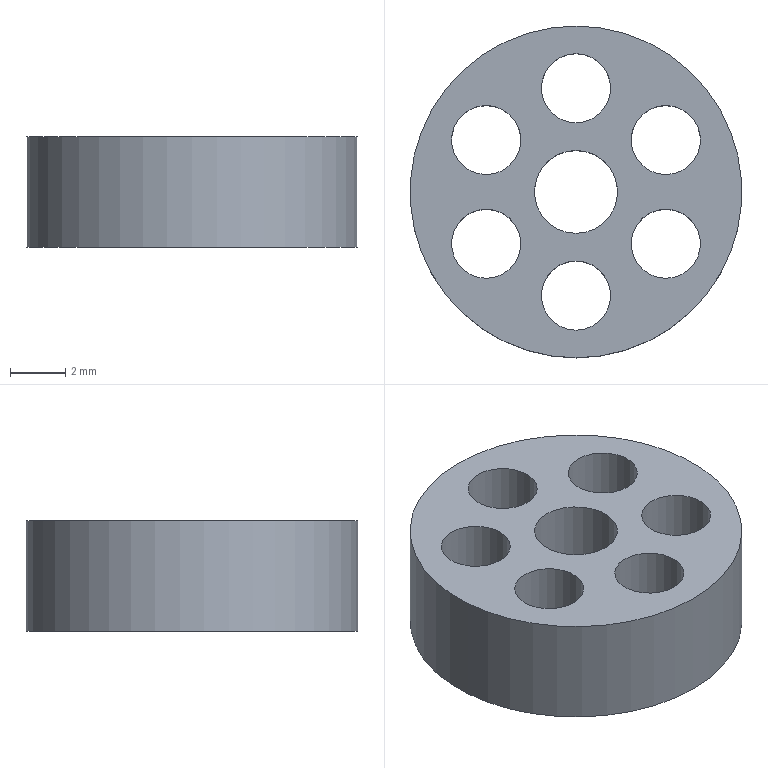Part | STEP file | 1-16.1 | 1 solid | 10 faces | box 12 x 12 x 4 mm | volume 306.305 mm3 | cylinder 8 | plane 2 | commonest cylinder face diameters 2.5 x6 3 x1 12 x1
STEP:
#1=CARTESIAN_POINT('',(0.,0.,0.));
#2=DIRECTION('',(0.,0.,1.));
#3=DIRECTION('',(1.,0.,0.));
#4=AXIS2_PLACEMENT_3D('',#1,#2,#3);
#5=CARTESIAN_POINT('',(0.,6.,0.));
#6=VERTEX_POINT('',#5);
#7=CARTESIAN_POINT('',(0.,0.,0.));
#8=DIRECTION('',(0.,0.,1.));
#9=DIRECTION('',(0.,1.,0.));
#10=AXIS2_PLACEMENT_3D('',#7,#8,#9);
#11=CIRCLE('',#10,6.);
#12=CARTESIAN_POINT('',(0.,-1.608,0.));
#13=DIRECTION('',(0.,0.,1.));
#14=DIRECTION('',(0.,1.,0.));
#15=AXIS2_PLACEMENT_3D('',#12,#13,#14);
#16=PLANE('',#15);
#17=CARTESIAN_POINT('',(1.608,0.));
#18=DIRECTION('',(1.,0.));
#19=AXIS2_PLACEMENT_2D('',#17,#18);
#20=CIRCLE('',#19,6.);
#21=(GEOMETRIC_REPRESENTATION_CONTEXT(2)PARAMETRIC_REPRESENTATION_CONTEXT()REPRESENTATION_CONTEXT('',''));
#22=DEFINITIONAL_REPRESENTATION('',(#20),#21);
#23=PCURVE('',#16,#22);
#24=CARTESIAN_POINT('',(0.,0.,0.));
#25=DIRECTION('',(0.,0.,1.));
#26=DIRECTION('',(0.,1.,0.));
#27=AXIS2_PLACEMENT_3D('',#24,#25,#26);
#28=CYLINDRICAL_SURFACE('',#27,6.);
#29=CARTESIAN_POINT('',(0.,0.));
#30=DIRECTION('',(1.,0.));
#31=VECTOR('',#30,1.);
#32=LINE('',#29,#31);
#33=(GEOMETRIC_REPRESENTATION_CONTEXT(2)PARAMETRIC_REPRESENTATION_CONTEXT()REPRESENTATION_CONTEXT('',''));
#34=DEFINITIONAL_REPRESENTATION('',(#32),#33);
#35=PCURVE('',#28,#34);
#36=SURFACE_CURVE('',#11,(#23,#35),.PCURVE_S1.);
#37=EDGE_CURVE('',#6,#6,#36,.T.);
#38=ORIENTED_EDGE('',*,*,#37,.T.);
#39=EDGE_LOOP('',(#38));
#40=FACE_BOUND('',#39,.F.);
#41=CARTESIAN_POINT('',(0.,5.,0.));
#42=VERTEX_POINT('',#41);
#43=CARTESIAN_POINT('',(0.,3.75,0.));
#44=DIRECTION('',(0.,0.,-1.));
#45=DIRECTION('',(0.,1.,0.));
#46=AXIS2_PLACEMENT_3D('',#43,#44,#45);
#47=CIRCLE('',#46,1.25);
#48=CARTESIAN_POINT('',(6.608,0.));
#49=CARTESIAN_POINT('',(6.608,-2.165));
#50=CARTESIAN_POINT('',(4.733,-1.083));
#51=CARTESIAN_POINT('',(2.858,0.));
#52=CARTESIAN_POINT('',(4.733,1.083));
#53=CARTESIAN_POINT('',(6.608,2.165));
#54=CARTESIAN_POINT('',(6.608,0.));
#55=(BOUNDED_CURVE()B_SPLINE_CURVE(2,(#48,#49,#50,#51,#52,#53,#54),.UNSPECIFIED.,.T.,.F.)B_SPLINE_CURVE_WITH_KNOTS((1,2,2,2,2,1),(-2.094,0.,2.094,4.189,6.283,8.378),.UNSPECIFIED.)CURVE()GEOMETRIC_REPRESENTATION_ITEM()RATIONAL_B_SPLINE_CURVE((1.,0.5,1.,0.5,1.,0.5,1.))REPRESENTATION_ITEM(''));
#56=(GEOMETRIC_REPRESENTATION_CONTEXT(2)PARAMETRIC_REPRESENTATION_CONTEXT()REPRESENTATION_CONTEXT('',''));
#57=DEFINITIONAL_REPRESENTATION('',(#55),#56);
#58=PCURVE('',#16,#57);
#59=CARTESIAN_POINT('',(0.,3.75,0.));
#60=DIRECTION('',(0.,0.,1.));
#61=DIRECTION('',(0.,1.,0.));
#62=AXIS2_PLACEMENT_3D('',#59,#60,#61);
#63=CYLINDRICAL_SURFACE('',#62,1.25);
#64=CARTESIAN_POINT('',(6.283,0.));
#65=DIRECTION('',(-1.,0.));
#66=VECTOR('',#65,1.);
#67=LINE('',#64,#66);
#68=(GEOMETRIC_REPRESENTATION_CONTEXT(2)PARAMETRIC_REPRESENTATION_CONTEXT()REPRESENTATION_CONTEXT('',''));
#69=DEFINITIONAL_REPRESENTATION('',(#67),#68);
#70=PCURVE('',#63,#69);
#71=SURFACE_CURVE('',#47,(#58,#70),.PCURVE_S1.);
#72=EDGE_CURVE('',#42,#42,#71,.T.);
#73=ORIENTED_EDGE('',*,*,#72,.T.);
#74=EDGE_LOOP('',(#73));
#75=FACE_BOUND('',#74,.F.);
#76=CARTESIAN_POINT('',(0.,1.5,0.));
#77=VERTEX_POINT('',#76);
#78=CARTESIAN_POINT('',(0.,0.,0.));
#79=DIRECTION('',(0.,0.,-1.));
#80=DIRECTION('',(0.,1.,0.));
#81=AXIS2_PLACEMENT_3D('',#78,#79,#80);
#82=CIRCLE('',#81,1.5);
#83=CARTESIAN_POINT('',(3.108,0.));
#84=CARTESIAN_POINT('',(3.108,-2.598));
#85=CARTESIAN_POINT('',(0.8577,-1.299));
#86=CARTESIAN_POINT('',(-1.392,0.));
#87=CARTESIAN_POINT('',(0.8577,1.299));
#88=CARTESIAN_POINT('',(3.108,2.598));
#89=CARTESIAN_POINT('',(3.108,0.));
#90=(BOUNDED_CURVE()B_SPLINE_CURVE(2,(#83,#84,#85,#86,#87,#88,#89),.UNSPECIFIED.,.T.,.F.)B_SPLINE_CURVE_WITH_KNOTS((1,2,2,2,2,1),(-2.094,0.,2.094,4.189,6.283,8.378),.UNSPECIFIED.)CURVE()GEOMETRIC_REPRESENTATION_ITEM()RATIONAL_B_SPLINE_CURVE((1.,0.5,1.,0.5,1.,0.5,1.))REPRESENTATION_ITEM(''));
#91=(GEOMETRIC_REPRESENTATION_CONTEXT(2)PARAMETRIC_REPRESENTATION_CONTEXT()REPRESENTATION_CONTEXT('',''));
#92=DEFINITIONAL_REPRESENTATION('',(#90),#91);
#93=PCURVE('',#16,#92);
#94=CARTESIAN_POINT('',(0.,0.,0.));
#95=DIRECTION('',(0.,0.,1.));
#96=DIRECTION('',(0.,1.,0.));
#97=AXIS2_PLACEMENT_3D('',#94,#95,#96);
#98=CYLINDRICAL_SURFACE('',#97,1.5);
#99=CARTESIAN_POINT('',(6.283,0.));
#100=DIRECTION('',(-1.,0.));
#101=VECTOR('',#100,1.);
#102=LINE('',#99,#101);
#103=(GEOMETRIC_REPRESENTATION_CONTEXT(2)PARAMETRIC_REPRESENTATION_CONTEXT()REPRESENTATION_CONTEXT('',''));
#104=DEFINITIONAL_REPRESENTATION('',(#102),#103);
#105=PCURVE('',#98,#104);
#106=SURFACE_CURVE('',#82,(#93,#105),.PCURVE_S1.);
#107=EDGE_CURVE('',#77,#77,#106,.T.);
#108=ORIENTED_EDGE('',*,*,#107,.T.);
#109=EDGE_LOOP('',(#108));
#110=FACE_BOUND('',#109,.F.);
#111=CARTESIAN_POINT('',(-3.248,3.125,0.));
#112=VERTEX_POINT('',#111);
#113=CARTESIAN_POINT('',(-3.248,1.875,0.));
#114=DIRECTION('',(0.,0.,-1.));
#115=DIRECTION('',(0.,1.,0.));
#116=AXIS2_PLACEMENT_3D('',#113,#114,#115);
#117=CIRCLE('',#116,1.25);
#118=CARTESIAN_POINT('',(4.733,3.248));
#119=CARTESIAN_POINT('',(4.733,1.083));
#120=CARTESIAN_POINT('',(2.858,2.165));
#121=CARTESIAN_POINT('',(0.9827,3.248));
#122=CARTESIAN_POINT('',(2.858,4.33));
#123=CARTESIAN_POINT('',(4.733,5.413));
#124=CARTESIAN_POINT('',(4.733,3.248));
#125=(BOUNDED_CURVE()B_SPLINE_CURVE(2,(#118,#119,#120,#121,#122,#123,#124),.UNSPECIFIED.,.T.,.F.)B_SPLINE_CURVE_WITH_KNOTS((1,2,2,2,2,1),(-2.094,0.,2.094,4.189,6.283,8.378),.UNSPECIFIED.)CURVE()GEOMETRIC_REPRESENTATION_ITEM()RATIONAL_B_SPLINE_CURVE((1.,0.5,1.,0.5,1.,0.5,1.))REPRESENTATION_ITEM(''));
#126=(GEOMETRIC_REPRESENTATION_CONTEXT(2)PARAMETRIC_REPRESENTATION_CONTEXT()REPRESENTATION_CONTEXT('',''));
#127=DEFINITIONAL_REPRESENTATION('',(#125),#126);
#128=PCURVE('',#16,#127);
#129=CARTESIAN_POINT('',(-3.248,1.875,0.));
#130=DIRECTION('',(0.,0.,1.));
#131=DIRECTION('',(0.,1.,0.));
#132=AXIS2_PLACEMENT_3D('',#129,#130,#131);
#133=CYLINDRICAL_SURFACE('',#132,1.25);
#134=CARTESIAN_POINT('',(6.283,0.));
#135=DIRECTION('',(-1.,0.));
#136=VECTOR('',#135,1.);
#137=LINE('',#134,#136);
#138=(GEOMETRIC_REPRESENTATION_CONTEXT(2)PARAMETRIC_REPRESENTATION_CONTEXT()REPRESENTATION_CONTEXT('',''));
#139=DEFINITIONAL_REPRESENTATION('',(#137),#138);
#140=PCURVE('',#133,#139);
#141=SURFACE_CURVE('',#117,(#128,#140),.PCURVE_S1.);
#142=EDGE_CURVE('',#112,#112,#141,.T.);
#143=ORIENTED_EDGE('',*,*,#142,.T.);
#144=EDGE_LOOP('',(#143));
#145=FACE_BOUND('',#144,.F.);
#146=CARTESIAN_POINT('',(-3.248,-0.625,0.));
#147=VERTEX_POINT('',#146);
#148=CARTESIAN_POINT('',(-3.248,-1.875,0.));
#149=DIRECTION('',(0.,0.,-1.));
#150=DIRECTION('',(0.,1.,0.));
#151=AXIS2_PLACEMENT_3D('',#148,#149,#150);
#152=CIRCLE('',#151,1.25);
#153=CARTESIAN_POINT('',(0.9827,3.248));
#154=CARTESIAN_POINT('',(0.9827,1.083));
#155=CARTESIAN_POINT('',(-0.8923,2.165));
#156=CARTESIAN_POINT('',(-2.767,3.248));
#157=CARTESIAN_POINT('',(-0.8923,4.33));
#158=CARTESIAN_POINT('',(0.9827,5.413));
#159=CARTESIAN_POINT('',(0.9827,3.248));
#160=(BOUNDED_CURVE()B_SPLINE_CURVE(2,(#153,#154,#155,#156,#157,#158,#159),.UNSPECIFIED.,.T.,.F.)B_SPLINE_CURVE_WITH_KNOTS((1,2,2,2,2,1),(-2.094,0.,2.094,4.189,6.283,8.378),.UNSPECIFIED.)CURVE()GEOMETRIC_REPRESENTATION_ITEM()RATIONAL_B_SPLINE_CURVE((1.,0.5,1.,0.5,1.,0.5,1.))REPRESENTATION_ITEM(''));
#161=(GEOMETRIC_REPRESENTATION_CONTEXT(2)PARAMETRIC_REPRESENTATION_CONTEXT()REPRESENTATION_CONTEXT('',''));
#162=DEFINITIONAL_REPRESENTATION('',(#160),#161);
#163=PCURVE('',#16,#162);
#164=CARTESIAN_POINT('',(-3.248,-1.875,0.));
#165=DIRECTION('',(0.,0.,1.));
#166=DIRECTION('',(0.,1.,0.));
#167=AXIS2_PLACEMENT_3D('',#164,#165,#166);
#168=CYLINDRICAL_SURFACE('',#167,1.25);
#169=CARTESIAN_POINT('',(6.283,0.));
#170=DIRECTION('',(-1.,0.));
#171=VECTOR('',#170,1.);
#172=LINE('',#169,#171);
#173=(GEOMETRIC_REPRESENTATION_CONTEXT(2)PARAMETRIC_REPRESENTATION_CONTEXT()REPRESENTATION_CONTEXT('',''));
#174=DEFINITIONAL_REPRESENTATION('',(#172),#173);
#175=PCURVE('',#168,#174);
#176=SURFACE_CURVE('',#152,(#163,#175),.PCURVE_S1.);
#177=EDGE_CURVE('',#147,#147,#176,.T.);
#178=ORIENTED_EDGE('',*,*,#177,.T.);
#179=EDGE_LOOP('',(#178));
#180=FACE_BOUND('',#179,.F.);
#181=CARTESIAN_POINT('',(0.,-2.5,0.));
#182=VERTEX_POINT('',#181);
#183=CARTESIAN_POINT('',(0.,-3.75,0.));
#184=DIRECTION('',(0.,0.,-1.));
#185=DIRECTION('',(0.,1.,0.));
#186=AXIS2_PLACEMENT_3D('',#183,#184,#185);
#187=CIRCLE('',#186,1.25);
#188=CARTESIAN_POINT('',(-0.8923,0.));
#189=CARTESIAN_POINT('',(-0.8923,-2.165));
#190=CARTESIAN_POINT('',(-2.767,-1.083));
#191=CARTESIAN_POINT('',(-4.642,0.));
#192=CARTESIAN_POINT('',(-2.767,1.083));
#193=CARTESIAN_POINT('',(-0.8923,2.165));
#194=CARTESIAN_POINT('',(-0.8923,0.));
#195=(BOUNDED_CURVE()B_SPLINE_CURVE(2,(#188,#189,#190,#191,#192,#193,#194),.UNSPECIFIED.,.T.,.F.)B_SPLINE_CURVE_WITH_KNOTS((1,2,2,2,2,1),(-2.094,0.,2.094,4.189,6.283,8.378),.UNSPECIFIED.)CURVE()GEOMETRIC_REPRESENTATION_ITEM()RATIONAL_B_SPLINE_CURVE((1.,0.5,1.,0.5,1.,0.5,1.))REPRESENTATION_ITEM(''));
#196=(GEOMETRIC_REPRESENTATION_CONTEXT(2)PARAMETRIC_REPRESENTATION_CONTEXT()REPRESENTATION_CONTEXT('',''));
#197=DEFINITIONAL_REPRESENTATION('',(#195),#196);
#198=PCURVE('',#16,#197);
#199=CARTESIAN_POINT('',(0.,-3.75,0.));
#200=DIRECTION('',(0.,0.,1.));
#201=DIRECTION('',(0.,1.,0.));
#202=AXIS2_PLACEMENT_3D('',#199,#200,#201);
#203=CYLINDRICAL_SURFACE('',#202,1.25);
#204=CARTESIAN_POINT('',(6.283,0.));
#205=DIRECTION('',(-1.,0.));
#206=VECTOR('',#205,1.);
#207=LINE('',#204,#206);
#208=(GEOMETRIC_REPRESENTATION_CONTEXT(2)PARAMETRIC_REPRESENTATION_CONTEXT()REPRESENTATION_CONTEXT('',''));
#209=DEFINITIONAL_REPRESENTATION('',(#207),#208);
#210=PCURVE('',#203,#209);
#211=SURFACE_CURVE('',#187,(#198,#210),.PCURVE_S1.);
#212=EDGE_CURVE('',#182,#182,#211,.T.);
#213=ORIENTED_EDGE('',*,*,#212,.T.);
#214=EDGE_LOOP('',(#213));
#215=FACE_BOUND('',#214,.F.);
#216=CARTESIAN_POINT('',(3.248,-0.625,0.));
#217=VERTEX_POINT('',#216);
#218=CARTESIAN_POINT('',(3.248,-1.875,0.));
#219=DIRECTION('',(0.,0.,-1.));
#220=DIRECTION('',(0.,1.,0.));
#221=AXIS2_PLACEMENT_3D('',#218,#219,#220);
#222=CIRCLE('',#221,1.25);
#223=CARTESIAN_POINT('',(0.9827,-3.248));
#224=CARTESIAN_POINT('',(0.9827,-5.413));
#225=CARTESIAN_POINT('',(-0.8923,-4.33));
#226=CARTESIAN_POINT('',(-2.767,-3.248));
#227=CARTESIAN_POINT('',(-0.8923,-2.165));
#228=CARTESIAN_POINT('',(0.9827,-1.083));
#229=CARTESIAN_POINT('',(0.9827,-3.248));
#230=(BOUNDED_CURVE()B_SPLINE_CURVE(2,(#223,#224,#225,#226,#227,#228,#229),.UNSPECIFIED.,.T.,.F.)B_SPLINE_CURVE_WITH_KNOTS((1,2,2,2,2,1),(-2.094,0.,2.094,4.189,6.283,8.378),.UNSPECIFIED.)CURVE()GEOMETRIC_REPRESENTATION_ITEM()RATIONAL_B_SPLINE_CURVE((1.,0.5,1.,0.5,1.,0.5,1.))REPRESENTATION_ITEM(''));
#231=(GEOMETRIC_REPRESENTATION_CONTEXT(2)PARAMETRIC_REPRESENTATION_CONTEXT()REPRESENTATION_CONTEXT('',''));
#232=DEFINITIONAL_REPRESENTATION('',(#230),#231);
#233=PCURVE('',#16,#232);
#234=CARTESIAN_POINT('',(3.248,-1.875,0.));
#235=DIRECTION('',(0.,0.,1.));
#236=DIRECTION('',(0.,1.,0.));
#237=AXIS2_PLACEMENT_3D('',#234,#235,#236);
#238=CYLINDRICAL_SURFACE('',#237,1.25);
#239=CARTESIAN_POINT('',(6.283,0.));
#240=DIRECTION('',(-1.,0.));
#241=VECTOR('',#240,1.);
#242=LINE('',#239,#241);
#243=(GEOMETRIC_REPRESENTATION_CONTEXT(2)PARAMETRIC_REPRESENTATION_CONTEXT()REPRESENTATION_CONTEXT('',''));
#244=DEFINITIONAL_REPRESENTATION('',(#242),#243);
#245=PCURVE('',#238,#244);
#246=SURFACE_CURVE('',#222,(#233,#245),.PCURVE_S1.);
#247=EDGE_CURVE('',#217,#217,#246,.T.);
#248=ORIENTED_EDGE('',*,*,#247,.T.);
#249=EDGE_LOOP('',(#248));
#250=FACE_BOUND('',#249,.F.);
#251=CARTESIAN_POINT('',(3.248,3.125,0.));
#252=VERTEX_POINT('',#251);
#253=CARTESIAN_POINT('',(3.248,1.875,0.));
#254=DIRECTION('',(0.,0.,-1.));
#255=DIRECTION('',(0.,1.,0.));
#256=AXIS2_PLACEMENT_3D('',#253,#254,#255);
#257=CIRCLE('',#256,1.25);
#258=CARTESIAN_POINT('',(4.733,-3.248));
#259=CARTESIAN_POINT('',(4.733,-5.413));
#260=CARTESIAN_POINT('',(2.858,-4.33));
#261=CARTESIAN_POINT('',(0.9827,-3.248));
#262=CARTESIAN_POINT('',(2.858,-2.165));
#263=CARTESIAN_POINT('',(4.733,-1.083));
#264=CARTESIAN_POINT('',(4.733,-3.248));
#265=(BOUNDED_CURVE()B_SPLINE_CURVE(2,(#258,#259,#260,#261,#262,#263,#264),.UNSPECIFIED.,.T.,.F.)B_SPLINE_CURVE_WITH_KNOTS((1,2,2,2,2,1),(-2.094,0.,2.094,4.189,6.283,8.378),.UNSPECIFIED.)CURVE()GEOMETRIC_REPRESENTATION_ITEM()RATIONAL_B_SPLINE_CURVE((1.,0.5,1.,0.5,1.,0.5,1.))REPRESENTATION_ITEM(''));
#266=(GEOMETRIC_REPRESENTATION_CONTEXT(2)PARAMETRIC_REPRESENTATION_CONTEXT()REPRESENTATION_CONTEXT('',''));
#267=DEFINITIONAL_REPRESENTATION('',(#265),#266);
#268=PCURVE('',#16,#267);
#269=CARTESIAN_POINT('',(3.248,1.875,0.));
#270=DIRECTION('',(0.,0.,1.));
#271=DIRECTION('',(0.,1.,0.));
#272=AXIS2_PLACEMENT_3D('',#269,#270,#271);
#273=CYLINDRICAL_SURFACE('',#272,1.25);
#274=CARTESIAN_POINT('',(6.283,0.));
#275=DIRECTION('',(-1.,0.));
#276=VECTOR('',#275,1.);
#277=LINE('',#274,#276);
#278=(GEOMETRIC_REPRESENTATION_CONTEXT(2)PARAMETRIC_REPRESENTATION_CONTEXT()REPRESENTATION_CONTEXT('',''));
#279=DEFINITIONAL_REPRESENTATION('',(#277),#278);
#280=PCURVE('',#273,#279);
#281=SURFACE_CURVE('',#257,(#268,#280),.PCURVE_S1.);
#282=EDGE_CURVE('',#252,#252,#281,.T.);
#283=ORIENTED_EDGE('',*,*,#282,.T.);
#284=EDGE_LOOP('',(#283));
#285=FACE_BOUND('',#284,.F.);
#286=ADVANCED_FACE('',(#40,#75,#110,#145,#180,#215,#250,#285),#16,.F.);
#287=CARTESIAN_POINT('',(0.,6.,4.));
#288=VERTEX_POINT('',#287);
#289=CARTESIAN_POINT('',(0.,0.,4.));
#290=DIRECTION('',(0.,0.,1.));
#291=DIRECTION('',(0.,1.,0.));
#292=AXIS2_PLACEMENT_3D('',#289,#290,#291);
#293=CIRCLE('',#292,6.);
#294=CARTESIAN_POINT('',(0.,-1.608,4.));
#295=DIRECTION('',(0.,0.,1.));
#296=DIRECTION('',(0.,1.,0.));
#297=AXIS2_PLACEMENT_3D('',#294,#295,#296);
#298=PLANE('',#297);
#299=CARTESIAN_POINT('',(1.608,0.));
#300=DIRECTION('',(1.,0.));
#301=AXIS2_PLACEMENT_2D('',#299,#300);
#302=CIRCLE('',#301,6.);
#303=(GEOMETRIC_REPRESENTATION_CONTEXT(2)PARAMETRIC_REPRESENTATION_CONTEXT()REPRESENTATION_CONTEXT('',''));
#304=DEFINITIONAL_REPRESENTATION('',(#302),#303);
#305=PCURVE('',#298,#304);
#306=CARTESIAN_POINT('',(0.,4.));
#307=DIRECTION('',(1.,0.));
#308=VECTOR('',#307,1.);
#309=LINE('',#306,#308);
#310=(GEOMETRIC_REPRESENTATION_CONTEXT(2)PARAMETRIC_REPRESENTATION_CONTEXT()REPRESENTATION_CONTEXT('',''));
#311=DEFINITIONAL_REPRESENTATION('',(#309),#310);
#312=PCURVE('',#28,#311);
#313=SURFACE_CURVE('',#293,(#305,#312),.PCURVE_S1.);
#314=EDGE_CURVE('',#288,#288,#313,.T.);
#315=ORIENTED_EDGE('',*,*,#314,.T.);
#316=EDGE_LOOP('',(#315));
#317=FACE_BOUND('',#316,.T.);
#318=CARTESIAN_POINT('',(0.,5.,4.));
#319=VERTEX_POINT('',#318);
#320=CARTESIAN_POINT('',(0.,3.75,4.));
#321=DIRECTION('',(0.,0.,-1.));
#322=DIRECTION('',(0.,1.,0.));
#323=AXIS2_PLACEMENT_3D('',#320,#321,#322);
#324=CIRCLE('',#323,1.25);
#325=CARTESIAN_POINT('',(6.608,0.));
#326=CARTESIAN_POINT('',(6.608,-2.165));
#327=CARTESIAN_POINT('',(4.733,-1.083));
#328=CARTESIAN_POINT('',(2.858,0.));
#329=CARTESIAN_POINT('',(4.733,1.083));
#330=CARTESIAN_POINT('',(6.608,2.165));
#331=CARTESIAN_POINT('',(6.608,0.));
#332=(BOUNDED_CURVE()B_SPLINE_CURVE(2,(#325,#326,#327,#328,#329,#330,#331),.UNSPECIFIED.,.T.,.F.)B_SPLINE_CURVE_WITH_KNOTS((1,2,2,2,2,1),(-2.094,0.,2.094,4.189,6.283,8.378),.UNSPECIFIED.)CURVE()GEOMETRIC_REPRESENTATION_ITEM()RATIONAL_B_SPLINE_CURVE((1.,0.5,1.,0.5,1.,0.5,1.))REPRESENTATION_ITEM(''));
#333=(GEOMETRIC_REPRESENTATION_CONTEXT(2)PARAMETRIC_REPRESENTATION_CONTEXT()REPRESENTATION_CONTEXT('',''));
#334=DEFINITIONAL_REPRESENTATION('',(#332),#333);
#335=PCURVE('',#298,#334);
#336=CARTESIAN_POINT('',(6.283,4.));
#337=DIRECTION('',(-1.,0.));
#338=VECTOR('',#337,1.);
#339=LINE('',#336,#338);
#340=(GEOMETRIC_REPRESENTATION_CONTEXT(2)PARAMETRIC_REPRESENTATION_CONTEXT()REPRESENTATION_CONTEXT('',''));
#341=DEFINITIONAL_REPRESENTATION('',(#339),#340);
#342=PCURVE('',#63,#341);
#343=SURFACE_CURVE('',#324,(#335,#342),.PCURVE_S1.);
#344=EDGE_CURVE('',#319,#319,#343,.T.);
#345=ORIENTED_EDGE('',*,*,#344,.T.);
#346=EDGE_LOOP('',(#345));
#347=FACE_BOUND('',#346,.T.);
#348=CARTESIAN_POINT('',(0.,1.5,4.));
#349=VERTEX_POINT('',#348);
#350=CARTESIAN_POINT('',(0.,0.,4.));
#351=DIRECTION('',(0.,0.,-1.));
#352=DIRECTION('',(0.,1.,0.));
#353=AXIS2_PLACEMENT_3D('',#350,#351,#352);
#354=CIRCLE('',#353,1.5);
#355=CARTESIAN_POINT('',(3.108,0.));
#356=CARTESIAN_POINT('',(3.108,-2.598));
#357=CARTESIAN_POINT('',(0.8577,-1.299));
#358=CARTESIAN_POINT('',(-1.392,0.));
#359=CARTESIAN_POINT('',(0.8577,1.299));
#360=CARTESIAN_POINT('',(3.108,2.598));
#361=CARTESIAN_POINT('',(3.108,0.));
#362=(BOUNDED_CURVE()B_SPLINE_CURVE(2,(#355,#356,#357,#358,#359,#360,#361),.UNSPECIFIED.,.T.,.F.)B_SPLINE_CURVE_WITH_KNOTS((1,2,2,2,2,1),(-2.094,0.,2.094,4.189,6.283,8.378),.UNSPECIFIED.)CURVE()GEOMETRIC_REPRESENTATION_ITEM()RATIONAL_B_SPLINE_CURVE((1.,0.5,1.,0.5,1.,0.5,1.))REPRESENTATION_ITEM(''));
#363=(GEOMETRIC_REPRESENTATION_CONTEXT(2)PARAMETRIC_REPRESENTATION_CONTEXT()REPRESENTATION_CONTEXT('',''));
#364=DEFINITIONAL_REPRESENTATION('',(#362),#363);
#365=PCURVE('',#298,#364);
#366=CARTESIAN_POINT('',(6.283,4.));
#367=DIRECTION('',(-1.,0.));
#368=VECTOR('',#367,1.);
#369=LINE('',#366,#368);
#370=(GEOMETRIC_REPRESENTATION_CONTEXT(2)PARAMETRIC_REPRESENTATION_CONTEXT()REPRESENTATION_CONTEXT('',''));
#371=DEFINITIONAL_REPRESENTATION('',(#369),#370);
#372=PCURVE('',#98,#371);
#373=SURFACE_CURVE('',#354,(#365,#372),.PCURVE_S1.);
#374=EDGE_CURVE('',#349,#349,#373,.T.);
#375=ORIENTED_EDGE('',*,*,#374,.T.);
#376=EDGE_LOOP('',(#375));
#377=FACE_BOUND('',#376,.T.);
#378=CARTESIAN_POINT('',(-3.248,3.125,4.));
#379=VERTEX_POINT('',#378);
#380=CARTESIAN_POINT('',(-3.248,1.875,4.));
#381=DIRECTION('',(0.,0.,-1.));
#382=DIRECTION('',(0.,1.,0.));
#383=AXIS2_PLACEMENT_3D('',#380,#381,#382);
#384=CIRCLE('',#383,1.25);
#385=CARTESIAN_POINT('',(4.733,3.248));
#386=CARTESIAN_POINT('',(4.733,1.083));
#387=CARTESIAN_POINT('',(2.858,2.165));
#388=CARTESIAN_POINT('',(0.9827,3.248));
#389=CARTESIAN_POINT('',(2.858,4.33));
#390=CARTESIAN_POINT('',(4.733,5.413));
#391=CARTESIAN_POINT('',(4.733,3.248));
#392=(BOUNDED_CURVE()B_SPLINE_CURVE(2,(#385,#386,#387,#388,#389,#390,#391),.UNSPECIFIED.,.T.,.F.)B_SPLINE_CURVE_WITH_KNOTS((1,2,2,2,2,1),(-2.094,0.,2.094,4.189,6.283,8.378),.UNSPECIFIED.)CURVE()GEOMETRIC_REPRESENTATION_ITEM()RATIONAL_B_SPLINE_CURVE((1.,0.5,1.,0.5,1.,0.5,1.))REPRESENTATION_ITEM(''));
#393=(GEOMETRIC_REPRESENTATION_CONTEXT(2)PARAMETRIC_REPRESENTATION_CONTEXT()REPRESENTATION_CONTEXT('',''));
#394=DEFINITIONAL_REPRESENTATION('',(#392),#393);
#395=PCURVE('',#298,#394);
#396=CARTESIAN_POINT('',(6.283,4.));
#397=DIRECTION('',(-1.,0.));
#398=VECTOR('',#397,1.);
#399=LINE('',#396,#398);
#400=(GEOMETRIC_REPRESENTATION_CONTEXT(2)PARAMETRIC_REPRESENTATION_CONTEXT()REPRESENTATION_CONTEXT('',''));
#401=DEFINITIONAL_REPRESENTATION('',(#399),#400);
#402=PCURVE('',#133,#401);
#403=SURFACE_CURVE('',#384,(#395,#402),.PCURVE_S1.);
#404=EDGE_CURVE('',#379,#379,#403,.T.);
#405=ORIENTED_EDGE('',*,*,#404,.T.);
#406=EDGE_LOOP('',(#405));
#407=FACE_BOUND('',#406,.T.);
#408=CARTESIAN_POINT('',(-3.248,-0.625,4.));
#409=VERTEX_POINT('',#408);
#410=CARTESIAN_POINT('',(-3.248,-1.875,4.));
#411=DIRECTION('',(0.,0.,-1.));
#412=DIRECTION('',(0.,1.,0.));
#413=AXIS2_PLACEMENT_3D('',#410,#411,#412);
#414=CIRCLE('',#413,1.25);
#415=CARTESIAN_POINT('',(0.9827,3.248));
#416=CARTESIAN_POINT('',(0.9827,1.083));
#417=CARTESIAN_POINT('',(-0.8923,2.165));
#418=CARTESIAN_POINT('',(-2.767,3.248));
#419=CARTESIAN_POINT('',(-0.8923,4.33));
#420=CARTESIAN_POINT('',(0.9827,5.413));
#421=CARTESIAN_POINT('',(0.9827,3.248));
#422=(BOUNDED_CURVE()B_SPLINE_CURVE(2,(#415,#416,#417,#418,#419,#420,#421),.UNSPECIFIED.,.T.,.F.)B_SPLINE_CURVE_WITH_KNOTS((1,2,2,2,2,1),(-2.094,0.,2.094,4.189,6.283,8.378),.UNSPECIFIED.)CURVE()GEOMETRIC_REPRESENTATION_ITEM()RATIONAL_B_SPLINE_CURVE((1.,0.5,1.,0.5,1.,0.5,1.))REPRESENTATION_ITEM(''));
#423=(GEOMETRIC_REPRESENTATION_CONTEXT(2)PARAMETRIC_REPRESENTATION_CONTEXT()REPRESENTATION_CONTEXT('',''));
#424=DEFINITIONAL_REPRESENTATION('',(#422),#423);
#425=PCURVE('',#298,#424);
#426=CARTESIAN_POINT('',(6.283,4.));
#427=DIRECTION('',(-1.,0.));
#428=VECTOR('',#427,1.);
#429=LINE('',#426,#428);
#430=(GEOMETRIC_REPRESENTATION_CONTEXT(2)PARAMETRIC_REPRESENTATION_CONTEXT()REPRESENTATION_CONTEXT('',''));
#431=DEFINITIONAL_REPRESENTATION('',(#429),#430);
#432=PCURVE('',#168,#431);
#433=SURFACE_CURVE('',#414,(#425,#432),.PCURVE_S1.);
#434=EDGE_CURVE('',#409,#409,#433,.T.);
#435=ORIENTED_EDGE('',*,*,#434,.T.);
#436=EDGE_LOOP('',(#435));
#437=FACE_BOUND('',#436,.T.);
#438=CARTESIAN_POINT('',(0.,-2.5,4.));
#439=VERTEX_POINT('',#438);
#440=CARTESIAN_POINT('',(0.,-3.75,4.));
#441=DIRECTION('',(0.,0.,-1.));
#442=DIRECTION('',(0.,1.,0.));
#443=AXIS2_PLACEMENT_3D('',#440,#441,#442);
#444=CIRCLE('',#443,1.25);
#445=CARTESIAN_POINT('',(-0.8923,0.));
#446=CARTESIAN_POINT('',(-0.8923,-2.165));
#447=CARTESIAN_POINT('',(-2.767,-1.083));
#448=CARTESIAN_POINT('',(-4.642,0.));
#449=CARTESIAN_POINT('',(-2.767,1.083));
#450=CARTESIAN_POINT('',(-0.8923,2.165));
#451=CARTESIAN_POINT('',(-0.8923,0.));
#452=(BOUNDED_CURVE()B_SPLINE_CURVE(2,(#445,#446,#447,#448,#449,#450,#451),.UNSPECIFIED.,.T.,.F.)B_SPLINE_CURVE_WITH_KNOTS((1,2,2,2,2,1),(-2.094,0.,2.094,4.189,6.283,8.378),.UNSPECIFIED.)CURVE()GEOMETRIC_REPRESENTATION_ITEM()RATIONAL_B_SPLINE_CURVE((1.,0.5,1.,0.5,1.,0.5,1.))REPRESENTATION_ITEM(''));
#453=(GEOMETRIC_REPRESENTATION_CONTEXT(2)PARAMETRIC_REPRESENTATION_CONTEXT()REPRESENTATION_CONTEXT('',''));
#454=DEFINITIONAL_REPRESENTATION('',(#452),#453);
#455=PCURVE('',#298,#454);
#456=CARTESIAN_POINT('',(6.283,4.));
#457=DIRECTION('',(-1.,0.));
#458=VECTOR('',#457,1.);
#459=LINE('',#456,#458);
#460=(GEOMETRIC_REPRESENTATION_CONTEXT(2)PARAMETRIC_REPRESENTATION_CONTEXT()REPRESENTATION_CONTEXT('',''));
#461=DEFINITIONAL_REPRESENTATION('',(#459),#460);
#462=PCURVE('',#203,#461);
#463=SURFACE_CURVE('',#444,(#455,#462),.PCURVE_S1.);
#464=EDGE_CURVE('',#439,#439,#463,.T.);
#465=ORIENTED_EDGE('',*,*,#464,.T.);
#466=EDGE_LOOP('',(#465));
#467=FACE_BOUND('',#466,.T.);
#468=CARTESIAN_POINT('',(3.248,-0.625,4.));
#469=VERTEX_POINT('',#468);
#470=CARTESIAN_POINT('',(3.248,-1.875,4.));
#471=DIRECTION('',(0.,0.,-1.));
#472=DIRECTION('',(0.,1.,0.));
#473=AXIS2_PLACEMENT_3D('',#470,#471,#472);
#474=CIRCLE('',#473,1.25);
#475=CARTESIAN_POINT('',(0.9827,-3.248));
#476=CARTESIAN_POINT('',(0.9827,-5.413));
#477=CARTESIAN_POINT('',(-0.8923,-4.33));
#478=CARTESIAN_POINT('',(-2.767,-3.248));
#479=CARTESIAN_POINT('',(-0.8923,-2.165));
#480=CARTESIAN_POINT('',(0.9827,-1.083));
#481=CARTESIAN_POINT('',(0.9827,-3.248));
#482=(BOUNDED_CURVE()B_SPLINE_CURVE(2,(#475,#476,#477,#478,#479,#480,#481),.UNSPECIFIED.,.T.,.F.)B_SPLINE_CURVE_WITH_KNOTS((1,2,2,2,2,1),(-2.094,0.,2.094,4.189,6.283,8.378),.UNSPECIFIED.)CURVE()GEOMETRIC_REPRESENTATION_ITEM()RATIONAL_B_SPLINE_CURVE((1.,0.5,1.,0.5,1.,0.5,1.))REPRESENTATION_ITEM(''));
#483=(GEOMETRIC_REPRESENTATION_CONTEXT(2)PARAMETRIC_REPRESENTATION_CONTEXT()REPRESENTATION_CONTEXT('',''));
#484=DEFINITIONAL_REPRESENTATION('',(#482),#483);
#485=PCURVE('',#298,#484);
#486=CARTESIAN_POINT('',(6.283,4.));
#487=DIRECTION('',(-1.,0.));
#488=VECTOR('',#487,1.);
#489=LINE('',#486,#488);
#490=(GEOMETRIC_REPRESENTATION_CONTEXT(2)PARAMETRIC_REPRESENTATION_CONTEXT()REPRESENTATION_CONTEXT('',''));
#491=DEFINITIONAL_REPRESENTATION('',(#489),#490);
#492=PCURVE('',#238,#491);
#493=SURFACE_CURVE('',#474,(#485,#492),.PCURVE_S1.);
#494=EDGE_CURVE('',#469,#469,#493,.T.);
#495=ORIENTED_EDGE('',*,*,#494,.T.);
#496=EDGE_LOOP('',(#495));
#497=FACE_BOUND('',#496,.T.);
#498=CARTESIAN_POINT('',(3.248,3.125,4.));
#499=VERTEX_POINT('',#498);
#500=CARTESIAN_POINT('',(3.248,1.875,4.));
#501=DIRECTION('',(0.,0.,-1.));
#502=DIRECTION('',(0.,1.,0.));
#503=AXIS2_PLACEMENT_3D('',#500,#501,#502);
#504=CIRCLE('',#503,1.25);
#505=CARTESIAN_POINT('',(4.733,-3.248));
#506=CARTESIAN_POINT('',(4.733,-5.413));
#507=CARTESIAN_POINT('',(2.858,-4.33));
#508=CARTESIAN_POINT('',(0.9827,-3.248));
#509=CARTESIAN_POINT('',(2.858,-2.165));
#510=CARTESIAN_POINT('',(4.733,-1.083));
#511=CARTESIAN_POINT('',(4.733,-3.248));
#512=(BOUNDED_CURVE()B_SPLINE_CURVE(2,(#505,#506,#507,#508,#509,#510,#511),.UNSPECIFIED.,.T.,.F.)B_SPLINE_CURVE_WITH_KNOTS((1,2,2,2,2,1),(-2.094,0.,2.094,4.189,6.283,8.378),.UNSPECIFIED.)CURVE()GEOMETRIC_REPRESENTATION_ITEM()RATIONAL_B_SPLINE_CURVE((1.,0.5,1.,0.5,1.,0.5,1.))REPRESENTATION_ITEM(''));
#513=(GEOMETRIC_REPRESENTATION_CONTEXT(2)PARAMETRIC_REPRESENTATION_CONTEXT()REPRESENTATION_CONTEXT('',''));
#514=DEFINITIONAL_REPRESENTATION('',(#512),#513);
#515=PCURVE('',#298,#514);
#516=CARTESIAN_POINT('',(6.283,4.));
#517=DIRECTION('',(-1.,0.));
#518=VECTOR('',#517,1.);
#519=LINE('',#516,#518);
#520=(GEOMETRIC_REPRESENTATION_CONTEXT(2)PARAMETRIC_REPRESENTATION_CONTEXT()REPRESENTATION_CONTEXT('',''));
#521=DEFINITIONAL_REPRESENTATION('',(#519),#520);
#522=PCURVE('',#273,#521);
#523=SURFACE_CURVE('',#504,(#515,#522),.PCURVE_S1.);
#524=EDGE_CURVE('',#499,#499,#523,.T.);
#525=ORIENTED_EDGE('',*,*,#524,.T.);
#526=EDGE_LOOP('',(#525));
#527=FACE_BOUND('',#526,.T.);
#528=ADVANCED_FACE('',(#317,#347,#377,#407,#437,#467,#497,#527),#298,.T.);
#529=ORIENTED_EDGE('',*,*,#37,.T.);
#530=CARTESIAN_POINT('',(0.,6.,0.));
#531=DIRECTION('',(0.,0.,1.));
#532=VECTOR('',#531,1.);
#533=LINE('',#530,#532);
#534=CARTESIAN_POINT('',(6.283,0.));
#535=DIRECTION('',(0.,1.));
#536=VECTOR('',#535,1.);
#537=LINE('',#534,#536);
#538=(GEOMETRIC_REPRESENTATION_CONTEXT(2)PARAMETRIC_REPRESENTATION_CONTEXT()REPRESENTATION_CONTEXT('',''));
#539=DEFINITIONAL_REPRESENTATION('',(#537),#538);
#540=PCURVE('',#28,#539);
#541=CARTESIAN_POINT('',(0.,0.));
#542=DIRECTION('',(0.,1.));
#543=VECTOR('',#542,1.);
#544=LINE('',#541,#543);
#545=(GEOMETRIC_REPRESENTATION_CONTEXT(2)PARAMETRIC_REPRESENTATION_CONTEXT()REPRESENTATION_CONTEXT('',''));
#546=DEFINITIONAL_REPRESENTATION('',(#544),#545);
#547=PCURVE('',#28,#546);
#548=SEAM_CURVE('',#533,(#540,#547),.PCURVE_S1.);
#549=EDGE_CURVE('',#6,#288,#548,.T.);
#550=ORIENTED_EDGE('',*,*,#549,.T.);
#551=ORIENTED_EDGE('',*,*,#314,.F.);
#552=ORIENTED_EDGE('',*,*,#549,.F.);
#553=EDGE_LOOP('',(#529,#550,#551,#552));
#554=FACE_BOUND('',#553,.T.);
#555=ADVANCED_FACE('',(#554),#28,.T.);
#556=CARTESIAN_POINT('',(0.,5.,0.));
#557=DIRECTION('',(0.,0.,1.));
#558=VECTOR('',#557,1.);
#559=LINE('',#556,#558);
#560=CARTESIAN_POINT('',(6.283,0.));
#561=DIRECTION('',(0.,1.));
#562=VECTOR('',#561,1.);
#563=LINE('',#560,#562);
#564=(GEOMETRIC_REPRESENTATION_CONTEXT(2)PARAMETRIC_REPRESENTATION_CONTEXT()REPRESENTATION_CONTEXT('',''));
#565=DEFINITIONAL_REPRESENTATION('',(#563),#564);
#566=PCURVE('',#63,#565);
#567=CARTESIAN_POINT('',(0.,0.));
#568=DIRECTION('',(0.,1.));
#569=VECTOR('',#568,1.);
#570=LINE('',#567,#569);
#571=(GEOMETRIC_REPRESENTATION_CONTEXT(2)PARAMETRIC_REPRESENTATION_CONTEXT()REPRESENTATION_CONTEXT('',''));
#572=DEFINITIONAL_REPRESENTATION('',(#570),#571);
#573=PCURVE('',#63,#572);
#574=SEAM_CURVE('',#559,(#566,#573),.PCURVE_S1.);
#575=EDGE_CURVE('',#42,#319,#574,.T.);
#576=ORIENTED_EDGE('',*,*,#575,.T.);
#577=ORIENTED_EDGE('',*,*,#344,.T.);
#578=ORIENTED_EDGE('',*,*,#575,.F.);
#579=ORIENTED_EDGE('',*,*,#72,.F.);
#580=EDGE_LOOP('',(#576,#577,#578,#579));
#581=FACE_BOUND('',#580,.F.);
#582=ADVANCED_FACE('',(#581),#63,.F.);
#583=CARTESIAN_POINT('',(0.,1.5,0.));
#584=DIRECTION('',(0.,0.,1.));
#585=VECTOR('',#584,1.);
#586=LINE('',#583,#585);
#587=CARTESIAN_POINT('',(6.283,0.));
#588=DIRECTION('',(0.,1.));
#589=VECTOR('',#588,1.);
#590=LINE('',#587,#589);
#591=(GEOMETRIC_REPRESENTATION_CONTEXT(2)PARAMETRIC_REPRESENTATION_CONTEXT()REPRESENTATION_CONTEXT('',''));
#592=DEFINITIONAL_REPRESENTATION('',(#590),#591);
#593=PCURVE('',#98,#592);
#594=CARTESIAN_POINT('',(0.,0.));
#595=DIRECTION('',(0.,1.));
#596=VECTOR('',#595,1.);
#597=LINE('',#594,#596);
#598=(GEOMETRIC_REPRESENTATION_CONTEXT(2)PARAMETRIC_REPRESENTATION_CONTEXT()REPRESENTATION_CONTEXT('',''));
#599=DEFINITIONAL_REPRESENTATION('',(#597),#598);
#600=PCURVE('',#98,#599);
#601=SEAM_CURVE('',#586,(#593,#600),.PCURVE_S1.);
#602=EDGE_CURVE('',#77,#349,#601,.T.);
#603=ORIENTED_EDGE('',*,*,#602,.T.);
#604=ORIENTED_EDGE('',*,*,#374,.T.);
#605=ORIENTED_EDGE('',*,*,#602,.F.);
#606=ORIENTED_EDGE('',*,*,#107,.F.);
#607=EDGE_LOOP('',(#603,#604,#605,#606));
#608=FACE_BOUND('',#607,.F.);
#609=ADVANCED_FACE('',(#608),#98,.F.);
#610=CARTESIAN_POINT('',(-3.248,3.125,0.));
#611=DIRECTION('',(0.,0.,1.));
#612=VECTOR('',#611,1.);
#613=LINE('',#610,#612);
#614=CARTESIAN_POINT('',(6.283,0.));
#615=DIRECTION('',(0.,1.));
#616=VECTOR('',#615,1.);
#617=LINE('',#614,#616);
#618=(GEOMETRIC_REPRESENTATION_CONTEXT(2)PARAMETRIC_REPRESENTATION_CONTEXT()REPRESENTATION_CONTEXT('',''));
#619=DEFINITIONAL_REPRESENTATION('',(#617),#618);
#620=PCURVE('',#133,#619);
#621=CARTESIAN_POINT('',(0.,0.));
#622=DIRECTION('',(0.,1.));
#623=VECTOR('',#622,1.);
#624=LINE('',#621,#623);
#625=(GEOMETRIC_REPRESENTATION_CONTEXT(2)PARAMETRIC_REPRESENTATION_CONTEXT()REPRESENTATION_CONTEXT('',''));
#626=DEFINITIONAL_REPRESENTATION('',(#624),#625);
#627=PCURVE('',#133,#626);
#628=SEAM_CURVE('',#613,(#620,#627),.PCURVE_S1.);
#629=EDGE_CURVE('',#112,#379,#628,.T.);
#630=ORIENTED_EDGE('',*,*,#629,.T.);
#631=ORIENTED_EDGE('',*,*,#404,.T.);
#632=ORIENTED_EDGE('',*,*,#629,.F.);
#633=ORIENTED_EDGE('',*,*,#142,.F.);
#634=EDGE_LOOP('',(#630,#631,#632,#633));
#635=FACE_BOUND('',#634,.F.);
#636=ADVANCED_FACE('',(#635),#133,.F.);
#637=CARTESIAN_POINT('',(-3.248,-0.625,0.));
#638=DIRECTION('',(0.,0.,1.));
#639=VECTOR('',#638,1.);
#640=LINE('',#637,#639);
#641=CARTESIAN_POINT('',(6.283,0.));
#642=DIRECTION('',(0.,1.));
#643=VECTOR('',#642,1.);
#644=LINE('',#641,#643);
#645=(GEOMETRIC_REPRESENTATION_CONTEXT(2)PARAMETRIC_REPRESENTATION_CONTEXT()REPRESENTATION_CONTEXT('',''));
#646=DEFINITIONAL_REPRESENTATION('',(#644),#645);
#647=PCURVE('',#168,#646);
#648=CARTESIAN_POINT('',(0.,0.));
#649=DIRECTION('',(0.,1.));
#650=VECTOR('',#649,1.);
#651=LINE('',#648,#650);
#652=(GEOMETRIC_REPRESENTATION_CONTEXT(2)PARAMETRIC_REPRESENTATION_CONTEXT()REPRESENTATION_CONTEXT('',''));
#653=DEFINITIONAL_REPRESENTATION('',(#651),#652);
#654=PCURVE('',#168,#653);
#655=SEAM_CURVE('',#640,(#647,#654),.PCURVE_S1.);
#656=EDGE_CURVE('',#147,#409,#655,.T.);
#657=ORIENTED_EDGE('',*,*,#656,.T.);
#658=ORIENTED_EDGE('',*,*,#434,.T.);
#659=ORIENTED_EDGE('',*,*,#656,.F.);
#660=ORIENTED_EDGE('',*,*,#177,.F.);
#661=EDGE_LOOP('',(#657,#658,#659,#660));
#662=FACE_BOUND('',#661,.F.);
#663=ADVANCED_FACE('',(#662),#168,.F.);
#664=CARTESIAN_POINT('',(0.,-2.5,0.));
#665=DIRECTION('',(0.,0.,1.));
#666=VECTOR('',#665,1.);
#667=LINE('',#664,#666);
#668=CARTESIAN_POINT('',(6.283,0.));
#669=DIRECTION('',(0.,1.));
#670=VECTOR('',#669,1.);
#671=LINE('',#668,#670);
#672=(GEOMETRIC_REPRESENTATION_CONTEXT(2)PARAMETRIC_REPRESENTATION_CONTEXT()REPRESENTATION_CONTEXT('',''));
#673=DEFINITIONAL_REPRESENTATION('',(#671),#672);
#674=PCURVE('',#203,#673);
#675=CARTESIAN_POINT('',(0.,0.));
#676=DIRECTION('',(0.,1.));
#677=VECTOR('',#676,1.);
#678=LINE('',#675,#677);
#679=(GEOMETRIC_REPRESENTATION_CONTEXT(2)PARAMETRIC_REPRESENTATION_CONTEXT()REPRESENTATION_CONTEXT('',''));
#680=DEFINITIONAL_REPRESENTATION('',(#678),#679);
#681=PCURVE('',#203,#680);
#682=SEAM_CURVE('',#667,(#674,#681),.PCURVE_S1.);
#683=EDGE_CURVE('',#182,#439,#682,.T.);
#684=ORIENTED_EDGE('',*,*,#683,.T.);
#685=ORIENTED_EDGE('',*,*,#464,.T.);
#686=ORIENTED_EDGE('',*,*,#683,.F.);
#687=ORIENTED_EDGE('',*,*,#212,.F.);
#688=EDGE_LOOP('',(#684,#685,#686,#687));
#689=FACE_BOUND('',#688,.F.);
#690=ADVANCED_FACE('',(#689),#203,.F.);
#691=CARTESIAN_POINT('',(3.248,-0.625,0.));
#692=DIRECTION('',(0.,0.,1.));
#693=VECTOR('',#692,1.);
#694=LINE('',#691,#693);
#695=CARTESIAN_POINT('',(6.283,0.));
#696=DIRECTION('',(0.,1.));
#697=VECTOR('',#696,1.);
#698=LINE('',#695,#697);
#699=(GEOMETRIC_REPRESENTATION_CONTEXT(2)PARAMETRIC_REPRESENTATION_CONTEXT()REPRESENTATION_CONTEXT('',''));
#700=DEFINITIONAL_REPRESENTATION('',(#698),#699);
#701=PCURVE('',#238,#700);
#702=CARTESIAN_POINT('',(0.,0.));
#703=DIRECTION('',(0.,1.));
#704=VECTOR('',#703,1.);
#705=LINE('',#702,#704);
#706=(GEOMETRIC_REPRESENTATION_CONTEXT(2)PARAMETRIC_REPRESENTATION_CONTEXT()REPRESENTATION_CONTEXT('',''));
#707=DEFINITIONAL_REPRESENTATION('',(#705),#706);
#708=PCURVE('',#238,#707);
#709=SEAM_CURVE('',#694,(#701,#708),.PCURVE_S1.);
#710=EDGE_CURVE('',#217,#469,#709,.T.);
#711=ORIENTED_EDGE('',*,*,#710,.T.);
#712=ORIENTED_EDGE('',*,*,#494,.T.);
#713=ORIENTED_EDGE('',*,*,#710,.F.);
#714=ORIENTED_EDGE('',*,*,#247,.F.);
#715=EDGE_LOOP('',(#711,#712,#713,#714));
#716=FACE_BOUND('',#715,.F.);
#717=ADVANCED_FACE('',(#716),#238,.F.);
#718=CARTESIAN_POINT('',(3.248,3.125,0.));
#719=DIRECTION('',(0.,0.,1.));
#720=VECTOR('',#719,1.);
#721=LINE('',#718,#720);
#722=CARTESIAN_POINT('',(6.283,0.));
#723=DIRECTION('',(0.,1.));
#724=VECTOR('',#723,1.);
#725=LINE('',#722,#724);
#726=(GEOMETRIC_REPRESENTATION_CONTEXT(2)PARAMETRIC_REPRESENTATION_CONTEXT()REPRESENTATION_CONTEXT('',''));
#727=DEFINITIONAL_REPRESENTATION('',(#725),#726);
#728=PCURVE('',#273,#727);
#729=CARTESIAN_POINT('',(0.,0.));
#730=DIRECTION('',(0.,1.));
#731=VECTOR('',#730,1.);
#732=LINE('',#729,#731);
#733=(GEOMETRIC_REPRESENTATION_CONTEXT(2)PARAMETRIC_REPRESENTATION_CONTEXT()REPRESENTATION_CONTEXT('',''));
#734=DEFINITIONAL_REPRESENTATION('',(#732),#733);
#735=PCURVE('',#273,#734);
#736=SEAM_CURVE('',#721,(#728,#735),.PCURVE_S1.);
#737=EDGE_CURVE('',#252,#499,#736,.T.);
#738=ORIENTED_EDGE('',*,*,#737,.T.);
#739=ORIENTED_EDGE('',*,*,#524,.T.);
#740=ORIENTED_EDGE('',*,*,#737,.F.);
#741=ORIENTED_EDGE('',*,*,#282,.F.);
#742=EDGE_LOOP('',(#738,#739,#740,#741));
#743=FACE_BOUND('',#742,.F.);
#744=ADVANCED_FACE('',(#743),#273,.F.);
#745=CLOSED_SHELL('',(#286,#528,#555,#582,#609,#636,#663,#690,#717,#744));
#746=MANIFOLD_SOLID_BREP('',#745);
#747=(LENGTH_UNIT()NAMED_UNIT(*)SI_UNIT(.MILLI.,.METRE.));
#748=UNCERTAINTY_MEASURE_WITH_UNIT(LENGTH_MEASURE(0.0000001),#747,'','');
#749=(NAMED_UNIT(*)PLANE_ANGLE_UNIT()SI_UNIT($,.RADIAN.));
#750=(NAMED_UNIT(*)SI_UNIT($,.STERADIAN.)SOLID_ANGLE_UNIT());
#751=(GEOMETRIC_REPRESENTATION_CONTEXT(3)GLOBAL_UNCERTAINTY_ASSIGNED_CONTEXT((#748))GLOBAL_UNIT_ASSIGNED_CONTEXT((#747,#749,#750))REPRESENTATION_CONTEXT('',''));
#752=ADVANCED_BREP_SHAPE_REPRESENTATION('',(#4,#746),#751);